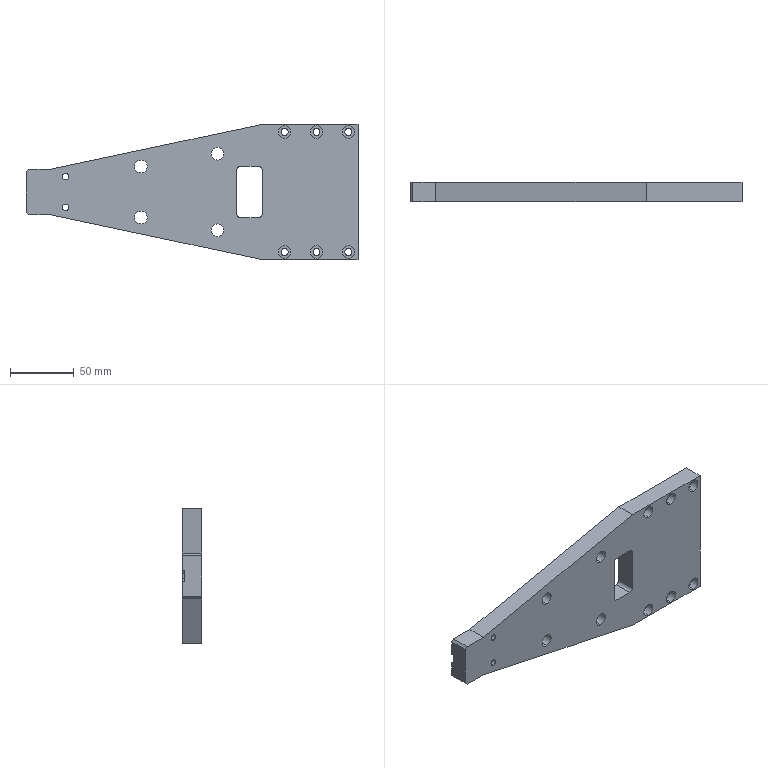Part | SolidWorks | features HoleWzd 4, ICE 2, Chamfer 1, Cut 1, Extrusion 1, Fillet 1 | 1 solid | 76 faces | box 260 x 15 x 106 mm | volume 283466 mm3 | cylinder 46 | plane 26 | cone 4 | commonest cylinder face diameters 10 x20 5.5 x12 2.5 x4 5 x4 6 x4 4 x2